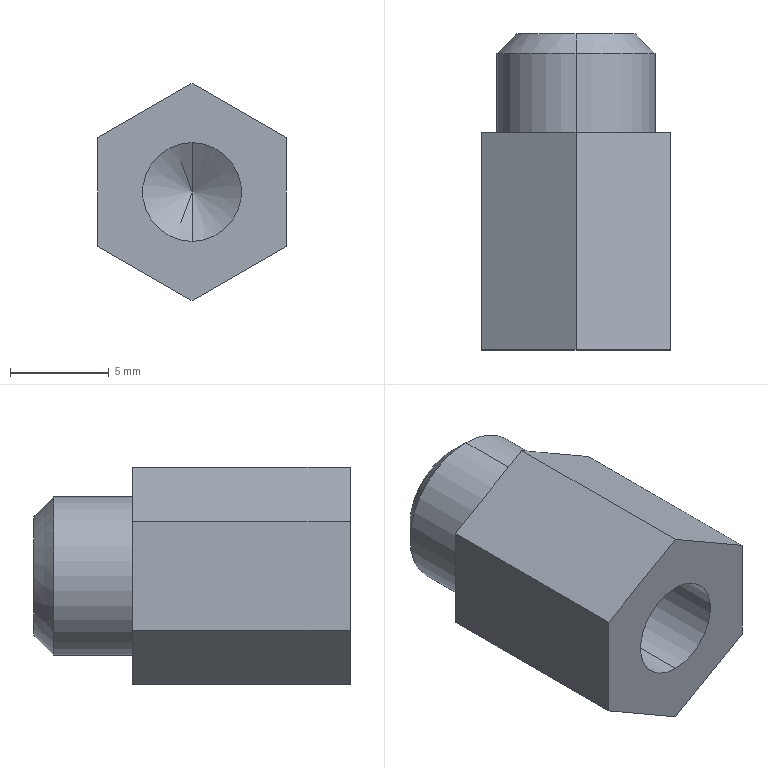Part | SolidWorks | features Chamfer 1, Extrusion 1, HoleWzd 1, ICE 1 | 1 solid | 17 faces | box 9.526 x 16 x 11 mm | volume 937.407 mm3 | plane 9 | cylinder 4 | cone 4 | commonest cylinder face diameters 5 x2 8 x2
STEP:
#1=CARTESIAN_POINT('',(0.001365,2.5,2.5));
#2=VERTEX_POINT('',#1);
#3=CARTESIAN_POINT('',(0.001365,2.5,-2.5));
#4=VERTEX_POINT('',#3);
#5=CARTESIAN_POINT('',(0.001365,2.5,0.));
#6=DIRECTION('',(0.,-1.,0.));
#7=DIRECTION('',(0.,0.,-1.));
#8=AXIS2_PLACEMENT_3D('',#5,#6,#7);
#9=CIRCLE('',#8,2.5);
#10=EDGE_CURVE('',#2,#4,#9,.T.);
#11=ORIENTED_EDGE('',*,*,#10,.F.);
#12=CARTESIAN_POINT('',(0.001365,-5.5,2.5));
#13=VERTEX_POINT('',#12);
#14=CARTESIAN_POINT('',(0.001365,-5.5,2.5));
#15=DIRECTION('',(0.,-1.,0.));
#16=VECTOR('',#15,1000.);
#17=LINE('',#14,#16);
#18=EDGE_CURVE('',#2,#13,#17,.T.);
#19=ORIENTED_EDGE('',*,*,#18,.T.);
#20=CARTESIAN_POINT('',(0.001365,-5.5,-2.5));
#21=VERTEX_POINT('',#20);
#22=CARTESIAN_POINT('',(0.001365,-5.5,0.));
#23=DIRECTION('',(0.,-1.,0.));
#24=DIRECTION('',(0.,0.,-1.));
#25=AXIS2_PLACEMENT_3D('',#22,#23,#24);
#26=CIRCLE('',#25,2.5);
#27=EDGE_CURVE('',#13,#21,#26,.T.);
#28=ORIENTED_EDGE('',*,*,#27,.T.);
#29=CARTESIAN_POINT('',(0.001365,-5.5,-2.5));
#30=DIRECTION('',(0.,-1.,0.));
#31=VECTOR('',#30,1000.);
#32=LINE('',#29,#31);
#33=EDGE_CURVE('',#4,#21,#32,.T.);
#34=ORIENTED_EDGE('',*,*,#33,.F.);
#35=EDGE_LOOP('',(#11,#19,#28,#34));
#36=FACE_OUTER_BOUND('',#35,.T.);
#37=CARTESIAN_POINT('',(0.001365,-5.5,0.));
#38=DIRECTION('',(0.,-1.,0.));
#39=DIRECTION('',(0.,0.,-1.));
#40=AXIS2_PLACEMENT_3D('',#37,#38,#39);
#41=CYLINDRICAL_SURFACE('',#40,2.5);
#42=ADVANCED_FACE('',(#36),#41,.F.);
#43=CARTESIAN_POINT('',(0.001365,4.002,0.));
#44=VERTEX_POINT('',#43);
#45=CARTESIAN_POINT('',(0.001365,2.5,-2.5));
#46=DIRECTION('',(0.,-0.515,-0.8572));
#47=VECTOR('',#46,1000.);
#48=LINE('',#45,#47);
#49=EDGE_CURVE('',#44,#4,#48,.T.);
#50=ORIENTED_EDGE('',*,*,#49,.F.);
#51=CARTESIAN_POINT('',(0.001365,2.5,2.5));
#52=DIRECTION('',(0.,-0.515,0.8572));
#53=VECTOR('',#52,1000.);
#54=LINE('',#51,#53);
#55=EDGE_CURVE('',#44,#2,#54,.T.);
#56=ORIENTED_EDGE('',*,*,#55,.T.);
#57=ORIENTED_EDGE('',*,*,#10,.T.);
#58=EDGE_LOOP('',(#50,#56,#57));
#59=FACE_OUTER_BOUND('',#58,.T.);
#60=CARTESIAN_POINT('',(0.001365,2.5,0.));
#61=DIRECTION('',(0.,-1.,0.));
#62=DIRECTION('',(0.,0.,-1.));
#63=AXIS2_PLACEMENT_3D('',#60,#61,#62);
#64=CONICAL_SURFACE('',#63,2.5,1.03);
#65=ADVANCED_FACE('',(#59),#64,.F.);
#66=CARTESIAN_POINT('',(0.,10.5,3.));
#67=VERTEX_POINT('',#66);
#68=CARTESIAN_POINT('',(0.,10.5,-3.));
#69=VERTEX_POINT('',#68);
#70=CARTESIAN_POINT('',(0.,10.5,0.));
#71=DIRECTION('',(0.,1.,0.));
#72=DIRECTION('',(0.,0.,1.));
#73=AXIS2_PLACEMENT_3D('',#70,#71,#72);
#74=CIRCLE('',#73,3.);
#75=EDGE_CURVE('',#67,#69,#74,.T.);
#76=ORIENTED_EDGE('',*,*,#75,.F.);
#77=CARTESIAN_POINT('',(0.,9.5,4.));
#78=VERTEX_POINT('',#77);
#79=CARTESIAN_POINT('',(0.,10.5,3.));
#80=DIRECTION('',(0.,-0.7071,0.7071));
#81=VECTOR('',#80,1000.);
#82=LINE('',#79,#81);
#83=EDGE_CURVE('',#67,#78,#82,.T.);
#84=ORIENTED_EDGE('',*,*,#83,.T.);
#85=CARTESIAN_POINT('',(0.,9.5,-4.));
#86=VERTEX_POINT('',#85);
#87=CARTESIAN_POINT('',(0.,9.5,0.));
#88=DIRECTION('',(0.,-1.,0.));
#89=DIRECTION('',(0.,0.,1.));
#90=AXIS2_PLACEMENT_3D('',#87,#88,#89);
#91=CIRCLE('',#90,4.);
#92=EDGE_CURVE('',#86,#78,#91,.T.);
#93=ORIENTED_EDGE('',*,*,#92,.F.);
#94=CARTESIAN_POINT('',(0.,10.5,-3.));
#95=DIRECTION('',(0.,-0.7071,-0.7071));
#96=VECTOR('',#95,1000.);
#97=LINE('',#94,#96);
#98=EDGE_CURVE('',#69,#86,#97,.T.);
#99=ORIENTED_EDGE('',*,*,#98,.F.);
#100=EDGE_LOOP('',(#76,#84,#93,#99));
#101=FACE_OUTER_BOUND('',#100,.T.);
#102=CARTESIAN_POINT('',(0.,10.5,0.));
#103=DIRECTION('',(0.,-1.,0.));
#104=DIRECTION('',(0.,0.,-1.));
#105=AXIS2_PLACEMENT_3D('',#102,#103,#104);
#106=CONICAL_SURFACE('',#105,3.,0.7854);
#107=ADVANCED_FACE('',(#101),#106,.T.);
#108=ORIENTED_EDGE('',*,*,#92,.T.);
#109=CARTESIAN_POINT('',(0.,5.5,4.));
#110=VERTEX_POINT('',#109);
#111=CARTESIAN_POINT('',(0.,10.5,4.));
#112=DIRECTION('',(0.,-1.,0.));
#113=VECTOR('',#112,1000.);
#114=LINE('',#111,#113);
#115=EDGE_CURVE('',#78,#110,#114,.T.);
#116=ORIENTED_EDGE('',*,*,#115,.T.);
#117=CARTESIAN_POINT('',(0.,5.5,-4.));
#118=VERTEX_POINT('',#117);
#119=CARTESIAN_POINT('',(0.,5.5,0.));
#120=DIRECTION('',(0.,1.,0.));
#121=DIRECTION('',(0.,0.,1.));
#122=AXIS2_PLACEMENT_3D('',#119,#120,#121);
#123=CIRCLE('',#122,4.);
#124=EDGE_CURVE('',#110,#118,#123,.T.);
#125=ORIENTED_EDGE('',*,*,#124,.T.);
#126=CARTESIAN_POINT('',(0.,10.5,-4.));
#127=DIRECTION('',(0.,-1.,0.));
#128=VECTOR('',#127,1000.);
#129=LINE('',#126,#128);
#130=EDGE_CURVE('',#86,#118,#129,.T.);
#131=ORIENTED_EDGE('',*,*,#130,.F.);
#132=EDGE_LOOP('',(#108,#116,#125,#131));
#133=FACE_OUTER_BOUND('',#132,.T.);
#134=CARTESIAN_POINT('',(0.,10.5,0.));
#135=DIRECTION('',(0.,-1.,0.));
#136=DIRECTION('',(0.,0.,-1.));
#137=AXIS2_PLACEMENT_3D('',#134,#135,#136);
#138=CYLINDRICAL_SURFACE('',#137,4.);
#139=ADVANCED_FACE('',(#133),#138,.T.);
#140=CARTESIAN_POINT('',(4.763,5.5,-2.75));
#141=VERTEX_POINT('',#140);
#142=CARTESIAN_POINT('',(0.,5.5,-5.5));
#143=VERTEX_POINT('',#142);
#144=CARTESIAN_POINT('',(4.763,5.5,-2.75));
#145=DIRECTION('',(-0.866,0.,-0.5));
#146=VECTOR('',#145,1000.);
#147=LINE('',#144,#146);
#148=EDGE_CURVE('',#141,#143,#147,.T.);
#149=ORIENTED_EDGE('',*,*,#148,.T.);
#150=CARTESIAN_POINT('',(-4.763,5.5,-2.75));
#151=VERTEX_POINT('',#150);
#152=CARTESIAN_POINT('',(0.,5.5,-5.5));
#153=DIRECTION('',(-0.866,0.,0.5));
#154=VECTOR('',#153,1000.);
#155=LINE('',#152,#154);
#156=EDGE_CURVE('',#143,#151,#155,.T.);
#157=ORIENTED_EDGE('',*,*,#156,.T.);
#158=CARTESIAN_POINT('',(-4.763,5.5,2.75));
#159=VERTEX_POINT('',#158);
#160=CARTESIAN_POINT('',(-4.763,5.5,-2.75));
#161=DIRECTION('',(0.,0.,1.));
#162=VECTOR('',#161,1000.);
#163=LINE('',#160,#162);
#164=EDGE_CURVE('',#151,#159,#163,.T.);
#165=ORIENTED_EDGE('',*,*,#164,.T.);
#166=CARTESIAN_POINT('',(0.,5.5,5.5));
#167=VERTEX_POINT('',#166);
#168=CARTESIAN_POINT('',(-4.763,5.5,2.75));
#169=DIRECTION('',(0.866,0.,0.5));
#170=VECTOR('',#169,1000.);
#171=LINE('',#168,#170);
#172=EDGE_CURVE('',#159,#167,#171,.T.);
#173=ORIENTED_EDGE('',*,*,#172,.T.);
#174=CARTESIAN_POINT('',(4.763,5.5,2.75));
#175=VERTEX_POINT('',#174);
#176=CARTESIAN_POINT('',(0.,5.5,5.5));
#177=DIRECTION('',(0.866,0.,-0.5));
#178=VECTOR('',#177,1000.);
#179=LINE('',#176,#178);
#180=EDGE_CURVE('',#167,#175,#179,.T.);
#181=ORIENTED_EDGE('',*,*,#180,.T.);
#182=CARTESIAN_POINT('',(4.763,5.5,2.75));
#183=DIRECTION('',(0.,0.,-1.));
#184=VECTOR('',#183,1000.);
#185=LINE('',#182,#184);
#186=EDGE_CURVE('',#175,#141,#185,.T.);
#187=ORIENTED_EDGE('',*,*,#186,.T.);
#188=EDGE_LOOP('',(#149,#157,#165,#173,#181,#187));
#189=FACE_OUTER_BOUND('',#188,.T.);
#190=CARTESIAN_POINT('',(0.,5.5,0.));
#191=DIRECTION('',(0.,1.,0.));
#192=DIRECTION('',(0.,0.,1.));
#193=AXIS2_PLACEMENT_3D('',#190,#191,#192);
#194=CIRCLE('',#193,4.);
#195=EDGE_CURVE('',#118,#110,#194,.T.);
#196=ORIENTED_EDGE('',*,*,#195,.F.);
#197=ORIENTED_EDGE('',*,*,#124,.F.);
#198=EDGE_LOOP('',(#196,#197));
#199=FACE_BOUND('',#198,.T.);
#200=CARTESIAN_POINT('',(0.,5.5,0.));
#201=DIRECTION('',(0.,1.,0.));
#202=DIRECTION('',(0.,0.,1.));
#203=AXIS2_PLACEMENT_3D('',#200,#201,#202);
#204=PLANE('',#203);
#205=ADVANCED_FACE('',(#189,#199),#204,.T.);
#206=CARTESIAN_POINT('',(4.763,-5.5,-2.75));
#207=VERTEX_POINT('',#206);
#208=CARTESIAN_POINT('',(0.,-5.5,-5.5));
#209=VERTEX_POINT('',#208);
#210=CARTESIAN_POINT('',(4.763,-5.5,-2.75));
#211=DIRECTION('',(-0.866,0.,-0.5));
#212=VECTOR('',#211,1000.);
#213=LINE('',#210,#212);
#214=EDGE_CURVE('',#207,#209,#213,.T.);
#215=ORIENTED_EDGE('',*,*,#214,.T.);
#216=CARTESIAN_POINT('',(0.,5.5,-5.5));
#217=DIRECTION('',(0.,-1.,0.));
#218=VECTOR('',#217,1000.);
#219=LINE('',#216,#218);
#220=EDGE_CURVE('',#143,#209,#219,.T.);
#221=ORIENTED_EDGE('',*,*,#220,.F.);
#222=ORIENTED_EDGE('',*,*,#148,.F.);
#223=CARTESIAN_POINT('',(4.763,5.5,-2.75));
#224=DIRECTION('',(0.,-1.,0.));
#225=VECTOR('',#224,1000.);
#226=LINE('',#223,#225);
#227=EDGE_CURVE('',#141,#207,#226,.T.);
#228=ORIENTED_EDGE('',*,*,#227,.T.);
#229=EDGE_LOOP('',(#215,#221,#222,#228));
#230=FACE_OUTER_BOUND('',#229,.T.);
#231=CARTESIAN_POINT('',(4.763,5.5,-2.75));
#232=DIRECTION('',(-0.5,0.,0.866));
#233=DIRECTION('',(0.866,0.,0.5));
#234=AXIS2_PLACEMENT_3D('',#231,#232,#233);
#235=PLANE('',#234);
#236=ADVANCED_FACE('',(#230),#235,.F.);
#237=CARTESIAN_POINT('',(-4.763,-5.5,-2.75));
#238=VERTEX_POINT('',#237);
#239=CARTESIAN_POINT('',(0.,-5.5,-5.5));
#240=DIRECTION('',(-0.866,0.,0.5));
#241=VECTOR('',#240,1000.);
#242=LINE('',#239,#241);
#243=EDGE_CURVE('',#209,#238,#242,.T.);
#244=ORIENTED_EDGE('',*,*,#243,.T.);
#245=CARTESIAN_POINT('',(-4.763,5.5,-2.75));
#246=DIRECTION('',(0.,-1.,0.));
#247=VECTOR('',#246,1000.);
#248=LINE('',#245,#247);
#249=EDGE_CURVE('',#151,#238,#248,.T.);
#250=ORIENTED_EDGE('',*,*,#249,.F.);
#251=ORIENTED_EDGE('',*,*,#156,.F.);
#252=ORIENTED_EDGE('',*,*,#220,.T.);
#253=EDGE_LOOP('',(#244,#250,#251,#252));
#254=FACE_OUTER_BOUND('',#253,.T.);
#255=CARTESIAN_POINT('',(0.,5.5,-5.5));
#256=DIRECTION('',(0.5,0.,0.866));
#257=DIRECTION('',(0.866,0.,-0.5));
#258=AXIS2_PLACEMENT_3D('',#255,#256,#257);
#259=PLANE('',#258);
#260=ADVANCED_FACE('',(#254),#259,.F.);
#261=CARTESIAN_POINT('',(-4.763,-5.5,2.75));
#262=VERTEX_POINT('',#261);
#263=CARTESIAN_POINT('',(-4.763,-5.5,-2.75));
#264=DIRECTION('',(0.,0.,1.));
#265=VECTOR('',#264,1000.);
#266=LINE('',#263,#265);
#267=EDGE_CURVE('',#238,#262,#266,.T.);
#268=ORIENTED_EDGE('',*,*,#267,.T.);
#269=CARTESIAN_POINT('',(-4.763,5.5,2.75));
#270=DIRECTION('',(0.,-1.,0.));
#271=VECTOR('',#270,1000.);
#272=LINE('',#269,#271);
#273=EDGE_CURVE('',#159,#262,#272,.T.);
#274=ORIENTED_EDGE('',*,*,#273,.F.);
#275=ORIENTED_EDGE('',*,*,#164,.F.);
#276=ORIENTED_EDGE('',*,*,#249,.T.);
#277=EDGE_LOOP('',(#268,#274,#275,#276));
#278=FACE_OUTER_BOUND('',#277,.T.);
#279=CARTESIAN_POINT('',(-4.763,5.5,-2.75));
#280=DIRECTION('',(1.,0.,0.));
#281=DIRECTION('',(0.,0.,-1.));
#282=AXIS2_PLACEMENT_3D('',#279,#280,#281);
#283=PLANE('',#282);
#284=ADVANCED_FACE('',(#278),#283,.F.);
#285=CARTESIAN_POINT('',(0.,-5.5,5.5));
#286=VERTEX_POINT('',#285);
#287=CARTESIAN_POINT('',(-4.763,-5.5,2.75));
#288=DIRECTION('',(0.866,0.,0.5));
#289=VECTOR('',#288,1000.);
#290=LINE('',#287,#289);
#291=EDGE_CURVE('',#262,#286,#290,.T.);
#292=ORIENTED_EDGE('',*,*,#291,.T.);
#293=CARTESIAN_POINT('',(0.,5.5,5.5));
#294=DIRECTION('',(0.,-1.,0.));
#295=VECTOR('',#294,1000.);
#296=LINE('',#293,#295);
#297=EDGE_CURVE('',#167,#286,#296,.T.);
#298=ORIENTED_EDGE('',*,*,#297,.F.);
#299=ORIENTED_EDGE('',*,*,#172,.F.);
#300=ORIENTED_EDGE('',*,*,#273,.T.);
#301=EDGE_LOOP('',(#292,#298,#299,#300));
#302=FACE_OUTER_BOUND('',#301,.T.);
#303=CARTESIAN_POINT('',(-4.763,5.5,2.75));
#304=DIRECTION('',(0.5,0.,-0.866));
#305=DIRECTION('',(-0.866,0.,-0.5));
#306=AXIS2_PLACEMENT_3D('',#303,#304,#305);
#307=PLANE('',#306);
#308=ADVANCED_FACE('',(#302),#307,.F.);
#309=CARTESIAN_POINT('',(4.763,-5.5,2.75));
#310=VERTEX_POINT('',#309);
#311=CARTESIAN_POINT('',(0.,-5.5,5.5));
#312=DIRECTION('',(0.866,0.,-0.5));
#313=VECTOR('',#312,1000.);
#314=LINE('',#311,#313);
#315=EDGE_CURVE('',#286,#310,#314,.T.);
#316=ORIENTED_EDGE('',*,*,#315,.T.);
#317=CARTESIAN_POINT('',(4.763,5.5,2.75));
#318=DIRECTION('',(0.,-1.,0.));
#319=VECTOR('',#318,1000.);
#320=LINE('',#317,#319);
#321=EDGE_CURVE('',#175,#310,#320,.T.);
#322=ORIENTED_EDGE('',*,*,#321,.F.);
#323=ORIENTED_EDGE('',*,*,#180,.F.);
#324=ORIENTED_EDGE('',*,*,#297,.T.);
#325=EDGE_LOOP('',(#316,#322,#323,#324));
#326=FACE_OUTER_BOUND('',#325,.T.);
#327=CARTESIAN_POINT('',(0.,5.5,5.5));
#328=DIRECTION('',(-0.5,0.,-0.866));
#329=DIRECTION('',(-0.866,0.,0.5));
#330=AXIS2_PLACEMENT_3D('',#327,#328,#329);
#331=PLANE('',#330);
#332=ADVANCED_FACE('',(#326),#331,.F.);
#333=CARTESIAN_POINT('',(4.763,-5.5,2.75));
#334=DIRECTION('',(0.,0.,-1.));
#335=VECTOR('',#334,1000.);
#336=LINE('',#333,#335);
#337=EDGE_CURVE('',#310,#207,#336,.T.);
#338=ORIENTED_EDGE('',*,*,#337,.T.);
#339=ORIENTED_EDGE('',*,*,#227,.F.);
#340=ORIENTED_EDGE('',*,*,#186,.F.);
#341=ORIENTED_EDGE('',*,*,#321,.T.);
#342=EDGE_LOOP('',(#338,#339,#340,#341));
#343=FACE_OUTER_BOUND('',#342,.T.);
#344=CARTESIAN_POINT('',(4.763,5.5,2.75));
#345=DIRECTION('',(-1.,0.,0.));
#346=DIRECTION('',(0.,0.,1.));
#347=AXIS2_PLACEMENT_3D('',#344,#345,#346);
#348=PLANE('',#347);
#349=ADVANCED_FACE('',(#343),#348,.F.);
#350=CARTESIAN_POINT('',(0.001365,-5.5,0.));
#351=DIRECTION('',(0.,-1.,0.));
#352=DIRECTION('',(0.,0.,-1.));
#353=AXIS2_PLACEMENT_3D('',#350,#351,#352);
#354=CIRCLE('',#353,2.5);
#355=EDGE_CURVE('',#21,#13,#354,.T.);
#356=ORIENTED_EDGE('',*,*,#355,.F.);
#357=ORIENTED_EDGE('',*,*,#27,.F.);
#358=EDGE_LOOP('',(#356,#357));
#359=FACE_BOUND('',#358,.T.);
#360=ORIENTED_EDGE('',*,*,#214,.F.);
#361=ORIENTED_EDGE('',*,*,#337,.F.);
#362=ORIENTED_EDGE('',*,*,#315,.F.);
#363=ORIENTED_EDGE('',*,*,#291,.F.);
#364=ORIENTED_EDGE('',*,*,#267,.F.);
#365=ORIENTED_EDGE('',*,*,#243,.F.);
#366=EDGE_LOOP('',(#360,#361,#362,#363,#364,#365));
#367=FACE_OUTER_BOUND('',#366,.T.);
#368=CARTESIAN_POINT('',(0.,-5.5,0.));
#369=DIRECTION('',(0.,1.,0.));
#370=DIRECTION('',(0.,0.,1.));
#371=AXIS2_PLACEMENT_3D('',#368,#369,#370);
#372=PLANE('',#371);
#373=ADVANCED_FACE('',(#359,#367),#372,.F.);
#374=ORIENTED_EDGE('',*,*,#115,.F.);
#375=CARTESIAN_POINT('',(0.,9.5,0.));
#376=DIRECTION('',(0.,-1.,0.));
#377=DIRECTION('',(0.,0.,1.));
#378=AXIS2_PLACEMENT_3D('',#375,#376,#377);
#379=CIRCLE('',#378,4.);
#380=EDGE_CURVE('',#78,#86,#379,.T.);
#381=ORIENTED_EDGE('',*,*,#380,.T.);
#382=ORIENTED_EDGE('',*,*,#130,.T.);
#383=ORIENTED_EDGE('',*,*,#195,.T.);
#384=EDGE_LOOP('',(#374,#381,#382,#383));
#385=FACE_OUTER_BOUND('',#384,.T.);
#386=CARTESIAN_POINT('',(0.,10.5,0.));
#387=DIRECTION('',(0.,-1.,0.));
#388=DIRECTION('',(0.,0.,-1.));
#389=AXIS2_PLACEMENT_3D('',#386,#387,#388);
#390=CYLINDRICAL_SURFACE('',#389,4.);
#391=ADVANCED_FACE('',(#385),#390,.T.);
#392=CARTESIAN_POINT('',(0.,10.5,0.));
#393=DIRECTION('',(0.,1.,0.));
#394=DIRECTION('',(0.,0.,1.));
#395=AXIS2_PLACEMENT_3D('',#392,#393,#394);
#396=CIRCLE('',#395,3.);
#397=EDGE_CURVE('',#69,#67,#396,.T.);
#398=ORIENTED_EDGE('',*,*,#397,.T.);
#399=ORIENTED_EDGE('',*,*,#75,.T.);
#400=EDGE_LOOP('',(#398,#399));
#401=FACE_OUTER_BOUND('',#400,.T.);
#402=CARTESIAN_POINT('',(0.,10.5,0.));
#403=DIRECTION('',(0.,1.,0.));
#404=DIRECTION('',(0.,0.,1.));
#405=AXIS2_PLACEMENT_3D('',#402,#403,#404);
#406=PLANE('',#405);
#407=ADVANCED_FACE('',(#401),#406,.T.);
#408=ORIENTED_EDGE('',*,*,#83,.F.);
#409=ORIENTED_EDGE('',*,*,#397,.F.);
#410=ORIENTED_EDGE('',*,*,#98,.T.);
#411=ORIENTED_EDGE('',*,*,#380,.F.);
#412=EDGE_LOOP('',(#408,#409,#410,#411));
#413=FACE_OUTER_BOUND('',#412,.T.);
#414=CARTESIAN_POINT('',(0.,10.5,0.));
#415=DIRECTION('',(0.,-1.,0.));
#416=DIRECTION('',(0.,0.,-1.));
#417=AXIS2_PLACEMENT_3D('',#414,#415,#416);
#418=CONICAL_SURFACE('',#417,3.,0.7854);
#419=ADVANCED_FACE('',(#413),#418,.T.);
#420=ORIENTED_EDGE('',*,*,#55,.F.);
#421=ORIENTED_EDGE('',*,*,#49,.T.);
#422=CARTESIAN_POINT('',(0.001365,2.5,0.));
#423=DIRECTION('',(0.,-1.,0.));
#424=DIRECTION('',(0.,0.,-1.));
#425=AXIS2_PLACEMENT_3D('',#422,#423,#424);
#426=CIRCLE('',#425,2.5);
#427=EDGE_CURVE('',#4,#2,#426,.T.);
#428=ORIENTED_EDGE('',*,*,#427,.T.);
#429=EDGE_LOOP('',(#420,#421,#428));
#430=FACE_OUTER_BOUND('',#429,.T.);
#431=CARTESIAN_POINT('',(0.001365,2.5,0.));
#432=DIRECTION('',(0.,-1.,0.));
#433=DIRECTION('',(0.,0.,-1.));
#434=AXIS2_PLACEMENT_3D('',#431,#432,#433);
#435=CONICAL_SURFACE('',#434,2.5,1.03);
#436=ADVANCED_FACE('',(#430),#435,.F.);
#437=ORIENTED_EDGE('',*,*,#18,.F.);
#438=ORIENTED_EDGE('',*,*,#427,.F.);
#439=ORIENTED_EDGE('',*,*,#33,.T.);
#440=ORIENTED_EDGE('',*,*,#355,.T.);
#441=EDGE_LOOP('',(#437,#438,#439,#440));
#442=FACE_OUTER_BOUND('',#441,.T.);
#443=CARTESIAN_POINT('',(0.001365,-5.5,0.));
#444=DIRECTION('',(0.,-1.,0.));
#445=DIRECTION('',(0.,0.,-1.));
#446=AXIS2_PLACEMENT_3D('',#443,#444,#445);
#447=CYLINDRICAL_SURFACE('',#446,2.5);
#448=ADVANCED_FACE('',(#442),#447,.F.);
#449=CLOSED_SHELL('',(#42,#65,#107,#139,#205,#236,#260,#284,#308,#332,#349,#373,#391,#407,#419,#436,#448));
#450=MANIFOLD_SOLID_BREP('',#449);
#451=CARTESIAN_POINT('',(0.,0.,0.));
#452=DIRECTION('',(0.,0.,1.));
#453=DIRECTION('',(1.,0.,0.));
#454=AXIS2_PLACEMENT_3D('',#451,#452,#453);
#455=(LENGTH_UNIT()NAMED_UNIT(*)SI_UNIT(.MILLI.,.METRE.));
#456=UNCERTAINTY_MEASURE_WITH_UNIT(LENGTH_MEASURE(0.00001),#455,'','');
#457=(NAMED_UNIT(*)PLANE_ANGLE_UNIT()SI_UNIT($,.RADIAN.));
#458=(NAMED_UNIT(*)SI_UNIT($,.STERADIAN.)SOLID_ANGLE_UNIT());
#459=(GEOMETRIC_REPRESENTATION_CONTEXT(3)GLOBAL_UNCERTAINTY_ASSIGNED_CONTEXT((#456))GLOBAL_UNIT_ASSIGNED_CONTEXT((#455,#457,#458))REPRESENTATION_CONTEXT('',''));
#460=ADVANCED_BREP_SHAPE_REPRESENTATION('',(#450,#454),#459);